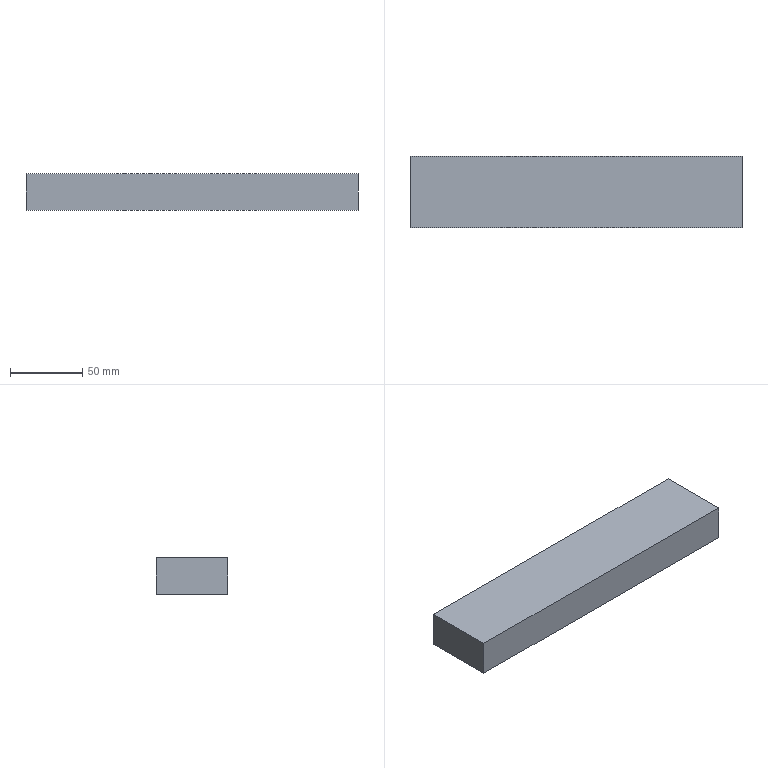Part | STEP file | 1 solid | 6 faces | box 229 x 49.201 x 25.123 mm | volume 283059 mm3 | plane 6
STEP:
#1=CARTESIAN_POINT('',(0.,0.,0.));
#2=DIRECTION('',(0.,0.,1.));
#3=DIRECTION('',(1.,0.,0.));
#4=AXIS2_PLACEMENT_3D('',#1,#2,#3);
#5=CARTESIAN_POINT('',(455.149,450.319,96.509));
#6=VERTEX_POINT('',#5);
#7=CARTESIAN_POINT('',(455.149,499.52,96.509));
#8=VERTEX_POINT('',#7);
#9=CARTESIAN_POINT('',(455.149,0.,96.509));
#10=DIRECTION('',(0.,1.,0.));
#11=VECTOR('',#10,1.);
#12=LINE('',#9,#11);
#13=CARTESIAN_POINT('',(226.149,0.,96.509));
#14=DIRECTION('',(0.,0.,-1.));
#15=DIRECTION('',(-1.,0.,0.));
#16=AXIS2_PLACEMENT_3D('',#13,#14,#15);
#17=PLANE('',#16);
#18=CARTESIAN_POINT('',(-229.,0.));
#19=DIRECTION('',(0.,1.));
#20=VECTOR('',#19,1.);
#21=LINE('',#18,#20);
#22=(GEOMETRIC_REPRESENTATION_CONTEXT(2)PARAMETRIC_REPRESENTATION_CONTEXT()REPRESENTATION_CONTEXT('',''));
#23=DEFINITIONAL_REPRESENTATION('',(#21),#22);
#24=PCURVE('',#17,#23);
#25=CARTESIAN_POINT('',(455.149,0.,0.));
#26=DIRECTION('',(-1.,0.,0.));
#27=DIRECTION('',(0.,0.,1.));
#28=AXIS2_PLACEMENT_3D('',#25,#26,#27);
#29=PLANE('',#28);
#30=CARTESIAN_POINT('',(96.509,0.));
#31=DIRECTION('',(0.,1.));
#32=VECTOR('',#31,1.);
#33=LINE('',#30,#32);
#34=(GEOMETRIC_REPRESENTATION_CONTEXT(2)PARAMETRIC_REPRESENTATION_CONTEXT()REPRESENTATION_CONTEXT('',''));
#35=DEFINITIONAL_REPRESENTATION('',(#33),#34);
#36=PCURVE('',#29,#35);
#37=SURFACE_CURVE('',#12,(#24,#36),.PCURVE_S1.);
#38=EDGE_CURVE('',#6,#8,#37,.T.);
#39=ORIENTED_EDGE('',*,*,#38,.F.);
#40=CARTESIAN_POINT('',(226.149,450.319,96.509));
#41=VERTEX_POINT('',#40);
#42=CARTESIAN_POINT('',(226.149,450.319,96.509));
#43=DIRECTION('',(1.,0.,0.));
#44=VECTOR('',#43,1.);
#45=LINE('',#42,#44);
#46=CARTESIAN_POINT('',(0.,450.319));
#47=DIRECTION('',(-1.,0.));
#48=VECTOR('',#47,1.);
#49=LINE('',#46,#48);
#50=(GEOMETRIC_REPRESENTATION_CONTEXT(2)PARAMETRIC_REPRESENTATION_CONTEXT()REPRESENTATION_CONTEXT('',''));
#51=DEFINITIONAL_REPRESENTATION('',(#49),#50);
#52=PCURVE('',#17,#51);
#53=CARTESIAN_POINT('',(226.149,450.319,0.));
#54=DIRECTION('',(0.,1.,0.));
#55=DIRECTION('',(0.,0.,1.));
#56=AXIS2_PLACEMENT_3D('',#53,#54,#55);
#57=PLANE('',#56);
#58=CARTESIAN_POINT('',(96.509,0.));
#59=DIRECTION('',(0.,1.));
#60=VECTOR('',#59,1.);
#61=LINE('',#58,#60);
#62=(GEOMETRIC_REPRESENTATION_CONTEXT(2)PARAMETRIC_REPRESENTATION_CONTEXT()REPRESENTATION_CONTEXT('',''));
#63=DEFINITIONAL_REPRESENTATION('',(#61),#62);
#64=PCURVE('',#57,#63);
#65=SURFACE_CURVE('',#45,(#52,#64),.PCURVE_S1.);
#66=EDGE_CURVE('',#41,#6,#65,.T.);
#67=ORIENTED_EDGE('',*,*,#66,.F.);
#68=CARTESIAN_POINT('',(226.149,499.52,96.509));
#69=VERTEX_POINT('',#68);
#70=CARTESIAN_POINT('',(226.149,0.,96.509));
#71=DIRECTION('',(0.,1.,0.));
#72=VECTOR('',#71,1.);
#73=LINE('',#70,#72);
#74=CARTESIAN_POINT('',(0.,0.));
#75=DIRECTION('',(0.,1.));
#76=VECTOR('',#75,1.);
#77=LINE('',#74,#76);
#78=(GEOMETRIC_REPRESENTATION_CONTEXT(2)PARAMETRIC_REPRESENTATION_CONTEXT()REPRESENTATION_CONTEXT('',''));
#79=DEFINITIONAL_REPRESENTATION('',(#77),#78);
#80=PCURVE('',#17,#79);
#81=CARTESIAN_POINT('',(226.149,0.,0.));
#82=DIRECTION('',(-1.,0.,0.));
#83=DIRECTION('',(0.,0.,1.));
#84=AXIS2_PLACEMENT_3D('',#81,#82,#83);
#85=PLANE('',#84);
#86=CARTESIAN_POINT('',(96.509,0.));
#87=DIRECTION('',(0.,1.));
#88=VECTOR('',#87,1.);
#89=LINE('',#86,#88);
#90=(GEOMETRIC_REPRESENTATION_CONTEXT(2)PARAMETRIC_REPRESENTATION_CONTEXT()REPRESENTATION_CONTEXT('',''));
#91=DEFINITIONAL_REPRESENTATION('',(#89),#90);
#92=PCURVE('',#85,#91);
#93=SURFACE_CURVE('',#73,(#80,#92),.PCURVE_S1.);
#94=EDGE_CURVE('',#41,#69,#93,.T.);
#95=ORIENTED_EDGE('',*,*,#94,.T.);
#96=CARTESIAN_POINT('',(226.149,499.52,96.509));
#97=DIRECTION('',(1.,0.,0.));
#98=VECTOR('',#97,1.);
#99=LINE('',#96,#98);
#100=CARTESIAN_POINT('',(0.,499.52));
#101=DIRECTION('',(-1.,0.));
#102=VECTOR('',#101,1.);
#103=LINE('',#100,#102);
#104=(GEOMETRIC_REPRESENTATION_CONTEXT(2)PARAMETRIC_REPRESENTATION_CONTEXT()REPRESENTATION_CONTEXT('',''));
#105=DEFINITIONAL_REPRESENTATION('',(#103),#104);
#106=PCURVE('',#17,#105);
#107=CARTESIAN_POINT('',(226.149,499.52,0.));
#108=DIRECTION('',(0.,-1.,0.));
#109=DIRECTION('',(0.,0.,-1.));
#110=AXIS2_PLACEMENT_3D('',#107,#108,#109);
#111=PLANE('',#110);
#112=CARTESIAN_POINT('',(-96.509,0.));
#113=DIRECTION('',(0.,1.));
#114=VECTOR('',#113,1.);
#115=LINE('',#112,#114);
#116=(GEOMETRIC_REPRESENTATION_CONTEXT(2)PARAMETRIC_REPRESENTATION_CONTEXT()REPRESENTATION_CONTEXT('',''));
#117=DEFINITIONAL_REPRESENTATION('',(#115),#116);
#118=PCURVE('',#111,#117);
#119=SURFACE_CURVE('',#99,(#106,#118),.PCURVE_S1.);
#120=EDGE_CURVE('',#69,#8,#119,.T.);
#121=ORIENTED_EDGE('',*,*,#120,.T.);
#122=EDGE_LOOP('',(#39,#67,#95,#121));
#123=FACE_BOUND('',#122,.T.);
#124=ADVANCED_FACE('',(#123),#17,.T.);
#125=CARTESIAN_POINT('',(455.149,450.319,121.632));
#126=VERTEX_POINT('',#125);
#127=CARTESIAN_POINT('',(455.149,450.319,0.));
#128=DIRECTION('',(0.,0.,1.));
#129=VECTOR('',#128,1.);
#130=LINE('',#127,#129);
#131=CARTESIAN_POINT('',(0.,229.));
#132=DIRECTION('',(1.,0.));
#133=VECTOR('',#132,1.);
#134=LINE('',#131,#133);
#135=(GEOMETRIC_REPRESENTATION_CONTEXT(2)PARAMETRIC_REPRESENTATION_CONTEXT()REPRESENTATION_CONTEXT('',''));
#136=DEFINITIONAL_REPRESENTATION('',(#134),#135);
#137=PCURVE('',#57,#136);
#138=CARTESIAN_POINT('',(0.,450.319));
#139=DIRECTION('',(1.,0.));
#140=VECTOR('',#139,1.);
#141=LINE('',#138,#140);
#142=(GEOMETRIC_REPRESENTATION_CONTEXT(2)PARAMETRIC_REPRESENTATION_CONTEXT()REPRESENTATION_CONTEXT('',''));
#143=DEFINITIONAL_REPRESENTATION('',(#141),#142);
#144=PCURVE('',#29,#143);
#145=SURFACE_CURVE('',#130,(#137,#144),.PCURVE_S1.);
#146=EDGE_CURVE('',#6,#126,#145,.T.);
#147=ORIENTED_EDGE('',*,*,#146,.T.);
#148=CARTESIAN_POINT('',(226.149,450.319,121.632));
#149=VERTEX_POINT('',#148);
#150=CARTESIAN_POINT('',(226.149,450.319,121.632));
#151=DIRECTION('',(1.,0.,0.));
#152=VECTOR('',#151,1.);
#153=LINE('',#150,#152);
#154=CARTESIAN_POINT('',(121.632,0.));
#155=DIRECTION('',(0.,1.));
#156=VECTOR('',#155,1.);
#157=LINE('',#154,#156);
#158=(GEOMETRIC_REPRESENTATION_CONTEXT(2)PARAMETRIC_REPRESENTATION_CONTEXT()REPRESENTATION_CONTEXT('',''));
#159=DEFINITIONAL_REPRESENTATION('',(#157),#158);
#160=PCURVE('',#57,#159);
#161=CARTESIAN_POINT('',(226.149,0.,121.632));
#162=DIRECTION('',(0.,0.,-1.));
#163=DIRECTION('',(-1.,0.,0.));
#164=AXIS2_PLACEMENT_3D('',#161,#162,#163);
#165=PLANE('',#164);
#166=CARTESIAN_POINT('',(0.,450.319));
#167=DIRECTION('',(-1.,0.));
#168=VECTOR('',#167,1.);
#169=LINE('',#166,#168);
#170=(GEOMETRIC_REPRESENTATION_CONTEXT(2)PARAMETRIC_REPRESENTATION_CONTEXT()REPRESENTATION_CONTEXT('',''));
#171=DEFINITIONAL_REPRESENTATION('',(#169),#170);
#172=PCURVE('',#165,#171);
#173=SURFACE_CURVE('',#153,(#160,#172),.PCURVE_S1.);
#174=EDGE_CURVE('',#149,#126,#173,.T.);
#175=ORIENTED_EDGE('',*,*,#174,.F.);
#176=CARTESIAN_POINT('',(226.149,450.319,0.));
#177=DIRECTION('',(0.,0.,1.));
#178=VECTOR('',#177,1.);
#179=LINE('',#176,#178);
#180=CARTESIAN_POINT('',(0.,0.));
#181=DIRECTION('',(1.,0.));
#182=VECTOR('',#181,1.);
#183=LINE('',#180,#182);
#184=(GEOMETRIC_REPRESENTATION_CONTEXT(2)PARAMETRIC_REPRESENTATION_CONTEXT()REPRESENTATION_CONTEXT('',''));
#185=DEFINITIONAL_REPRESENTATION('',(#183),#184);
#186=PCURVE('',#57,#185);
#187=CARTESIAN_POINT('',(0.,450.319));
#188=DIRECTION('',(1.,0.));
#189=VECTOR('',#188,1.);
#190=LINE('',#187,#189);
#191=(GEOMETRIC_REPRESENTATION_CONTEXT(2)PARAMETRIC_REPRESENTATION_CONTEXT()REPRESENTATION_CONTEXT('',''));
#192=DEFINITIONAL_REPRESENTATION('',(#190),#191);
#193=PCURVE('',#85,#192);
#194=SURFACE_CURVE('',#179,(#186,#193),.PCURVE_S1.);
#195=EDGE_CURVE('',#41,#149,#194,.T.);
#196=ORIENTED_EDGE('',*,*,#195,.F.);
#197=ORIENTED_EDGE('',*,*,#66,.T.);
#198=EDGE_LOOP('',(#147,#175,#196,#197));
#199=FACE_BOUND('',#198,.T.);
#200=ADVANCED_FACE('',(#199),#57,.F.);
#201=CARTESIAN_POINT('',(455.149,499.52,121.632));
#202=VERTEX_POINT('',#201);
#203=CARTESIAN_POINT('',(455.149,0.,121.632));
#204=DIRECTION('',(0.,1.,0.));
#205=VECTOR('',#204,1.);
#206=LINE('',#203,#205);
#207=CARTESIAN_POINT('',(-229.,0.));
#208=DIRECTION('',(0.,1.));
#209=VECTOR('',#208,1.);
#210=LINE('',#207,#209);
#211=(GEOMETRIC_REPRESENTATION_CONTEXT(2)PARAMETRIC_REPRESENTATION_CONTEXT()REPRESENTATION_CONTEXT('',''));
#212=DEFINITIONAL_REPRESENTATION('',(#210),#211);
#213=PCURVE('',#165,#212);
#214=CARTESIAN_POINT('',(121.632,0.));
#215=DIRECTION('',(0.,1.));
#216=VECTOR('',#215,1.);
#217=LINE('',#214,#216);
#218=(GEOMETRIC_REPRESENTATION_CONTEXT(2)PARAMETRIC_REPRESENTATION_CONTEXT()REPRESENTATION_CONTEXT('',''));
#219=DEFINITIONAL_REPRESENTATION('',(#217),#218);
#220=PCURVE('',#29,#219);
#221=SURFACE_CURVE('',#206,(#213,#220),.PCURVE_S1.);
#222=EDGE_CURVE('',#126,#202,#221,.T.);
#223=ORIENTED_EDGE('',*,*,#222,.T.);
#224=CARTESIAN_POINT('',(226.149,499.52,121.632));
#225=VERTEX_POINT('',#224);
#226=CARTESIAN_POINT('',(226.149,499.52,121.632));
#227=DIRECTION('',(1.,0.,0.));
#228=VECTOR('',#227,1.);
#229=LINE('',#226,#228);
#230=CARTESIAN_POINT('',(0.,499.52));
#231=DIRECTION('',(-1.,0.));
#232=VECTOR('',#231,1.);
#233=LINE('',#230,#232);
#234=(GEOMETRIC_REPRESENTATION_CONTEXT(2)PARAMETRIC_REPRESENTATION_CONTEXT()REPRESENTATION_CONTEXT('',''));
#235=DEFINITIONAL_REPRESENTATION('',(#233),#234);
#236=PCURVE('',#165,#235);
#237=CARTESIAN_POINT('',(-121.632,0.));
#238=DIRECTION('',(0.,1.));
#239=VECTOR('',#238,1.);
#240=LINE('',#237,#239);
#241=(GEOMETRIC_REPRESENTATION_CONTEXT(2)PARAMETRIC_REPRESENTATION_CONTEXT()REPRESENTATION_CONTEXT('',''));
#242=DEFINITIONAL_REPRESENTATION('',(#240),#241);
#243=PCURVE('',#111,#242);
#244=SURFACE_CURVE('',#229,(#236,#243),.PCURVE_S1.);
#245=EDGE_CURVE('',#225,#202,#244,.T.);
#246=ORIENTED_EDGE('',*,*,#245,.F.);
#247=CARTESIAN_POINT('',(226.149,0.,121.632));
#248=DIRECTION('',(0.,1.,0.));
#249=VECTOR('',#248,1.);
#250=LINE('',#247,#249);
#251=CARTESIAN_POINT('',(0.,0.));
#252=DIRECTION('',(0.,1.));
#253=VECTOR('',#252,1.);
#254=LINE('',#251,#253);
#255=(GEOMETRIC_REPRESENTATION_CONTEXT(2)PARAMETRIC_REPRESENTATION_CONTEXT()REPRESENTATION_CONTEXT('',''));
#256=DEFINITIONAL_REPRESENTATION('',(#254),#255);
#257=PCURVE('',#165,#256);
#258=CARTESIAN_POINT('',(121.632,0.));
#259=DIRECTION('',(0.,1.));
#260=VECTOR('',#259,1.);
#261=LINE('',#258,#260);
#262=(GEOMETRIC_REPRESENTATION_CONTEXT(2)PARAMETRIC_REPRESENTATION_CONTEXT()REPRESENTATION_CONTEXT('',''));
#263=DEFINITIONAL_REPRESENTATION('',(#261),#262);
#264=PCURVE('',#85,#263);
#265=SURFACE_CURVE('',#250,(#257,#264),.PCURVE_S1.);
#266=EDGE_CURVE('',#149,#225,#265,.T.);
#267=ORIENTED_EDGE('',*,*,#266,.F.);
#268=ORIENTED_EDGE('',*,*,#174,.T.);
#269=EDGE_LOOP('',(#223,#246,#267,#268));
#270=FACE_BOUND('',#269,.T.);
#271=ADVANCED_FACE('',(#270),#165,.F.);
#272=CARTESIAN_POINT('',(455.149,499.52,0.));
#273=DIRECTION('',(0.,0.,-1.));
#274=VECTOR('',#273,1.);
#275=LINE('',#272,#274);
#276=CARTESIAN_POINT('',(0.,229.));
#277=DIRECTION('',(1.,0.));
#278=VECTOR('',#277,1.);
#279=LINE('',#276,#278);
#280=(GEOMETRIC_REPRESENTATION_CONTEXT(2)PARAMETRIC_REPRESENTATION_CONTEXT()REPRESENTATION_CONTEXT('',''));
#281=DEFINITIONAL_REPRESENTATION('',(#279),#280);
#282=PCURVE('',#111,#281);
#283=CARTESIAN_POINT('',(0.,499.52));
#284=DIRECTION('',(-1.,0.));
#285=VECTOR('',#284,1.);
#286=LINE('',#283,#285);
#287=(GEOMETRIC_REPRESENTATION_CONTEXT(2)PARAMETRIC_REPRESENTATION_CONTEXT()REPRESENTATION_CONTEXT('',''));
#288=DEFINITIONAL_REPRESENTATION('',(#286),#287);
#289=PCURVE('',#29,#288);
#290=SURFACE_CURVE('',#275,(#282,#289),.PCURVE_S1.);
#291=EDGE_CURVE('',#202,#8,#290,.T.);
#292=ORIENTED_EDGE('',*,*,#291,.T.);
#293=ORIENTED_EDGE('',*,*,#120,.F.);
#294=CARTESIAN_POINT('',(226.149,499.52,0.));
#295=DIRECTION('',(0.,0.,-1.));
#296=VECTOR('',#295,1.);
#297=LINE('',#294,#296);
#298=CARTESIAN_POINT('',(0.,0.));
#299=DIRECTION('',(1.,0.));
#300=VECTOR('',#299,1.);
#301=LINE('',#298,#300);
#302=(GEOMETRIC_REPRESENTATION_CONTEXT(2)PARAMETRIC_REPRESENTATION_CONTEXT()REPRESENTATION_CONTEXT('',''));
#303=DEFINITIONAL_REPRESENTATION('',(#301),#302);
#304=PCURVE('',#111,#303);
#305=CARTESIAN_POINT('',(0.,499.52));
#306=DIRECTION('',(-1.,0.));
#307=VECTOR('',#306,1.);
#308=LINE('',#305,#307);
#309=(GEOMETRIC_REPRESENTATION_CONTEXT(2)PARAMETRIC_REPRESENTATION_CONTEXT()REPRESENTATION_CONTEXT('',''));
#310=DEFINITIONAL_REPRESENTATION('',(#308),#309);
#311=PCURVE('',#85,#310);
#312=SURFACE_CURVE('',#297,(#304,#311),.PCURVE_S1.);
#313=EDGE_CURVE('',#225,#69,#312,.T.);
#314=ORIENTED_EDGE('',*,*,#313,.F.);
#315=ORIENTED_EDGE('',*,*,#245,.T.);
#316=EDGE_LOOP('',(#292,#293,#314,#315));
#317=FACE_BOUND('',#316,.T.);
#318=ADVANCED_FACE('',(#317),#111,.F.);
#319=ORIENTED_EDGE('',*,*,#94,.F.);
#320=ORIENTED_EDGE('',*,*,#195,.T.);
#321=ORIENTED_EDGE('',*,*,#266,.T.);
#322=ORIENTED_EDGE('',*,*,#313,.T.);
#323=EDGE_LOOP('',(#319,#320,#321,#322));
#324=FACE_BOUND('',#323,.T.);
#325=ADVANCED_FACE('',(#324),#85,.T.);
#326=ORIENTED_EDGE('',*,*,#38,.T.);
#327=ORIENTED_EDGE('',*,*,#291,.F.);
#328=ORIENTED_EDGE('',*,*,#222,.F.);
#329=ORIENTED_EDGE('',*,*,#146,.F.);
#330=EDGE_LOOP('',(#326,#327,#328,#329));
#331=FACE_BOUND('',#330,.T.);
#332=ADVANCED_FACE('',(#331),#29,.F.);
#333=CLOSED_SHELL('',(#124,#200,#271,#318,#325,#332));
#334=MANIFOLD_SOLID_BREP('',#333);
#335=(LENGTH_UNIT()NAMED_UNIT(*)SI_UNIT(.MILLI.,.METRE.));
#336=UNCERTAINTY_MEASURE_WITH_UNIT(LENGTH_MEASURE(0.0000001),#335,'','');
#337=(NAMED_UNIT(*)PLANE_ANGLE_UNIT()SI_UNIT($,.RADIAN.));
#338=(NAMED_UNIT(*)SI_UNIT($,.STERADIAN.)SOLID_ANGLE_UNIT());
#339=(GEOMETRIC_REPRESENTATION_CONTEXT(3)GLOBAL_UNCERTAINTY_ASSIGNED_CONTEXT((#336))GLOBAL_UNIT_ASSIGNED_CONTEXT((#335,#337,#338))REPRESENTATION_CONTEXT('',''));
#340=ADVANCED_BREP_SHAPE_REPRESENTATION('',(#4,#334),#339);